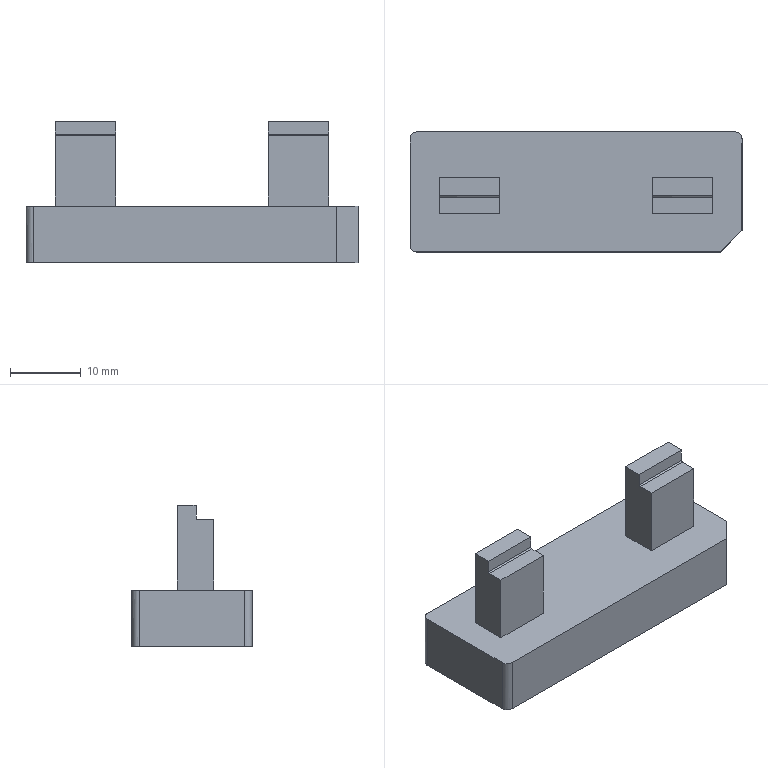CAM job | PowerMill | 3-axis milling, other | part box 47 x 17 x 19.985 mm
Tools:
number,name,type,diameter,tip_radius,length,cutting_length,overhang,flutes,holder,toolpaths_using
1,D10C,end_mill,10.0,0.0,60.0,,30.0,1,D42L35,1
14,D4_2,end_mill,4.0,0.0,30.0,,12.16,1,D42L35,2
1,D10C_1_1_1,end_mill,10.0,0.0,60.0,,20.44,1,D42L35,3
2,D4C_1_1,end_mill,4.0,0.0,30.0,,12.16,1,D42L35,1
3,D10_1_1_1,end_mill,10.0,0.0,60.0,,20.16,1,D42L35,3
13,Text_D4_1_1,taper_spherical,4.0,0.3,60.0,,12.24,1,D42L35,1
Operations:
program,toolpath,strategy,tool,tool_number,tool_diameter,tip_radius,flutes,spindle_rpm,feed_cut,surface_speed_m_min_computed,feed_per_tooth_computed,tolerance,thickness,stepover,stepdown,cut_length,cut_time_min,total_time_min,workplane
07-0518-1-F,精公开粗01-扫面平行-D10C,raster_area_clear,D10C_1_1_1,1,10.0,0.0,1.0,8000.0,10000.0,251.33,1.25,0.03,0.28,6.0,1.0,285.36,0.029,0.035,
07-0518-1-F,精公开粗01-外形偏置-D10C,offset_area_clear,D10C_1_1_1,1,10.0,0.0,1.0,8000.0,10000.0,251.33,1.25,0.03,0.28,6.0,1.0,9472.265,0.947,1.024,
07-0518-1-F,精公开粗01-基准台等高-D10C,constantz,D10C_1_1_1,1,10.0,0.0,1.0,8000.0,10000.0,251.33,1.25,0.03,0.07,5.0,0.4,3449.083,0.345,0.3552,
07-0518-1-F,精公再粗02-外形偏置-D4C,offset_area_clear,D4C_1_1,2,4.0,0.0,1.0,18000.0,6000.0,226.19,0.3333,0.03,0.0,2.0,1.0,5233.278,0.872,0.9581,
07-0518-1-F,精公基准台01-平坦面偏置-D10,offset_area_clear,D10_1_1_1,3,10.0,0.0,1.0,8500.0,600.0,267.04,0.0706,0.005,0.38,5.0,1.0,114.782,0.191,0.2527,
07-0518-1-F,精公基准台01-基准面偏置-D10,offset_area_clear,D10_1_1_1,3,10.0,0.0,1.0,8500.0,600.0,267.04,0.0706,0.005,0.38,5.0,1.0,195.35,0.326,0.3668,
07-0518-1-F,精公基准台01-基准台侧光-D10,profile_area_clear,D10_1_1_1,3,10.0,0.0,1.0,8500.0,600.0,267.04,0.0706,0.005,0.0,0.08,1.0,313.234,0.522,0.5869,
07-0518-1-F,精公精光01-等高-D4,constantz,D4_2,14,4.0,0.0,1.0,18000.0,2000.0,226.19,0.1111,0.005,-0.075,5.0,0.1,9299.511,4.65,5.059,
07-0518-1-F,精公精光01-平坦面平行-D4,raster_area_clear,D4_2,14,4.0,0.0,1.0,18000.0,600.0,226.19,0.0333,0.005,0.375,2.0,1.0,155.583,0.259,0.3224,
07-0518-1-F,精公刻字01-刻字-Text_D4,pattern,Text_D4_1_1,13,4.0,0.3,1.0,15000.0,1000.0,188.5,0.0667,0.005,0.0,5.0,1.0,66.497,0.067,0.0887,
,精公开粗01-外形偏置-D10C_Reference,offset_area_clear,D10C,1,10.0,0.0,1.0,8000.0,10000.0,251.33,1.25,0.03,0.28,6.0,1.0,18944.562,1.894,2.044,